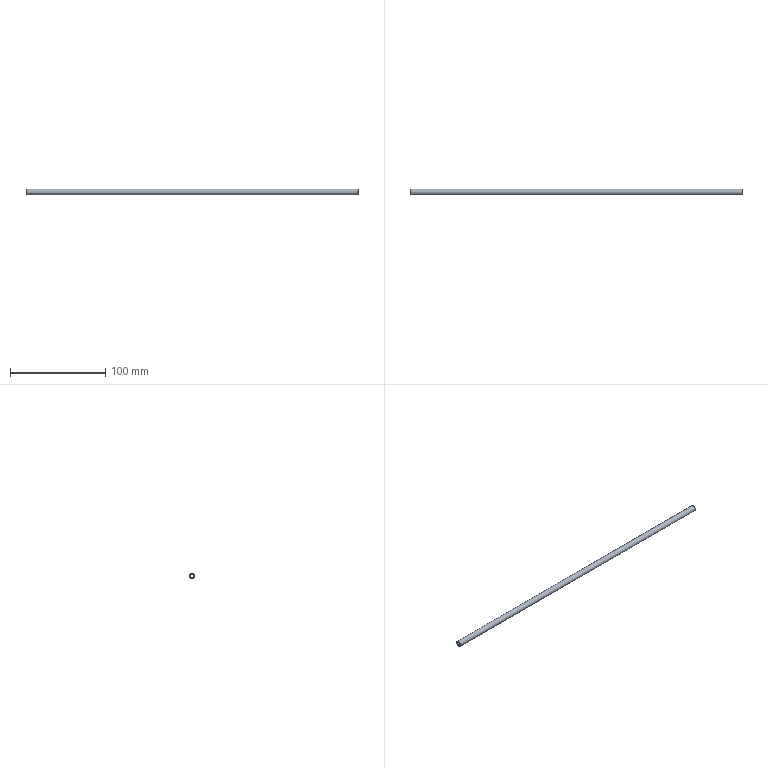Part | NX | features solid 2 | 1 solid | 4 faces | box 348.824 x 6 x 6 mm | volume 5479 mm3 | cylinder 2 | plane 2 | commonest cylinder face diameters 4 x1 6 x1
STEP:
#1=CARTESIAN_POINT('',(-423.824,-82.,347.));
#2=VERTEX_POINT('',#1);
#3=CARTESIAN_POINT('',(-423.824,-80.,347.));
#4=DIRECTION('',(-1.,0.,0.));
#5=DIRECTION('',(0.,-1.,0.));
#6=AXIS2_PLACEMENT_3D('',#3,#4,#5);
#7=CIRCLE('',#6,2.);
#8=EDGE_CURVE('',#2,#2,#7,.T.);
#9=ORIENTED_EDGE('',*,*,#8,.T.);
#10=EDGE_LOOP('',(#9));
#11=FACE_BOUND('',#10,.T.);
#12=CARTESIAN_POINT('',(-75.,-82.,347.));
#13=VERTEX_POINT('',#12);
#14=CARTESIAN_POINT('',(-75.,-80.,347.));
#15=DIRECTION('',(-1.,0.,0.));
#16=DIRECTION('',(0.,-1.,0.));
#17=AXIS2_PLACEMENT_3D('',#14,#15,#16);
#18=CIRCLE('',#17,2.);
#19=EDGE_CURVE('',#13,#13,#18,.T.);
#20=ORIENTED_EDGE('',*,*,#19,.F.);
#21=EDGE_LOOP('',(#20));
#22=FACE_BOUND('',#21,.T.);
#23=CARTESIAN_POINT('',(-273.824,-80.,347.));
#24=DIRECTION('',(1.,0.,0.));
#25=DIRECTION('',(0.,1.,0.));
#26=AXIS2_PLACEMENT_3D('',#23,#24,#25);
#27=CYLINDRICAL_SURFACE('',#26,2.);
#28=ADVANCED_FACE('',(#11,#22),#27,.F.);
#29=CARTESIAN_POINT('',(-423.824,-83.,347.));
#30=VERTEX_POINT('',#29);
#31=CARTESIAN_POINT('',(-423.824,-80.,347.));
#32=DIRECTION('',(-1.,0.,0.));
#33=DIRECTION('',(0.,-1.,0.));
#34=AXIS2_PLACEMENT_3D('',#31,#32,#33);
#35=CIRCLE('',#34,3.);
#36=EDGE_CURVE('',#30,#30,#35,.T.);
#37=ORIENTED_EDGE('',*,*,#36,.F.);
#38=EDGE_LOOP('',(#37));
#39=FACE_BOUND('',#38,.T.);
#40=CARTESIAN_POINT('',(-75.,-83.,347.));
#41=VERTEX_POINT('',#40);
#42=CARTESIAN_POINT('',(-75.,-80.,347.));
#43=DIRECTION('',(-1.,0.,0.));
#44=DIRECTION('',(0.,-1.,0.));
#45=AXIS2_PLACEMENT_3D('',#42,#43,#44);
#46=CIRCLE('',#45,3.);
#47=EDGE_CURVE('',#41,#41,#46,.T.);
#48=ORIENTED_EDGE('',*,*,#47,.T.);
#49=EDGE_LOOP('',(#48));
#50=FACE_BOUND('',#49,.T.);
#51=CARTESIAN_POINT('',(-273.824,-80.,347.));
#52=DIRECTION('',(1.,0.,0.));
#53=DIRECTION('',(0.,1.,0.));
#54=AXIS2_PLACEMENT_3D('',#51,#52,#53);
#55=CYLINDRICAL_SURFACE('',#54,3.);
#56=ADVANCED_FACE('',(#39,#50),#55,.T.);
#57=ORIENTED_EDGE('',*,*,#8,.F.);
#58=EDGE_LOOP('',(#57));
#59=FACE_BOUND('',#58,.T.);
#60=ORIENTED_EDGE('',*,*,#36,.T.);
#61=EDGE_LOOP('',(#60));
#62=FACE_BOUND('',#61,.T.);
#63=CARTESIAN_POINT('',(-423.824,-80.,347.));
#64=DIRECTION('',(-1.,0.,0.));
#65=DIRECTION('',(0.,-1.,0.));
#66=AXIS2_PLACEMENT_3D('',#63,#64,#65);
#67=PLANE('',#66);
#68=ADVANCED_FACE('',(#59,#62),#67,.T.);
#69=ORIENTED_EDGE('',*,*,#19,.T.);
#70=EDGE_LOOP('',(#69));
#71=FACE_BOUND('',#70,.T.);
#72=ORIENTED_EDGE('',*,*,#47,.F.);
#73=EDGE_LOOP('',(#72));
#74=FACE_BOUND('',#73,.T.);
#75=CARTESIAN_POINT('',(-75.,-80.,347.));
#76=DIRECTION('',(-1.,0.,0.));
#77=DIRECTION('',(0.,-1.,0.));
#78=AXIS2_PLACEMENT_3D('',#75,#76,#77);
#79=PLANE('',#78);
#80=ADVANCED_FACE('',(#71,#74),#79,.F.);
#81=CLOSED_SHELL('',(#28,#56,#68,#80));
#82=MANIFOLD_SOLID_BREP('',#81);
#83=(LENGTH_UNIT()NAMED_UNIT(*)SI_UNIT(.MILLI.,.METRE.));
#84=UNCERTAINTY_MEASURE_WITH_UNIT(LENGTH_MEASURE(0.00001),#83,'','');
#85=(NAMED_UNIT(*)PLANE_ANGLE_UNIT()SI_UNIT($,.RADIAN.));
#86=(NAMED_UNIT(*)SI_UNIT($,.STERADIAN.)SOLID_ANGLE_UNIT());
#87=(GEOMETRIC_REPRESENTATION_CONTEXT(3)GLOBAL_UNCERTAINTY_ASSIGNED_CONTEXT((#84))GLOBAL_UNIT_ASSIGNED_CONTEXT((#83,#85,#86))REPRESENTATION_CONTEXT('',''));
#88=ADVANCED_BREP_SHAPE_REPRESENTATION('',(#82),#87);